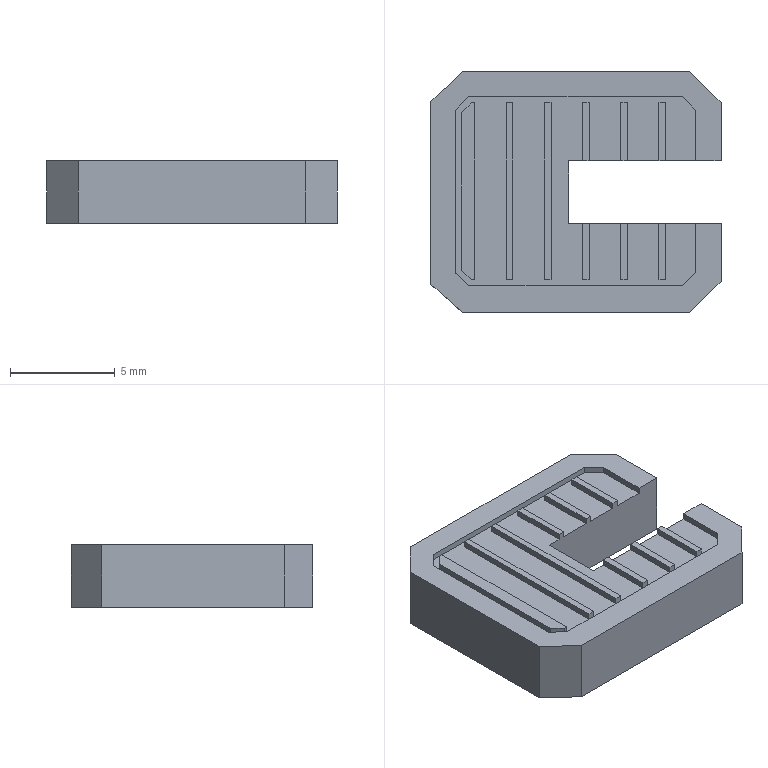Part | SolidWorks | features BaseBody 1 | 1 solid | 65 faces | box 13.855 x 11.523 x 3 mm | volume 379.654 mm3 | plane 62 | spline 3